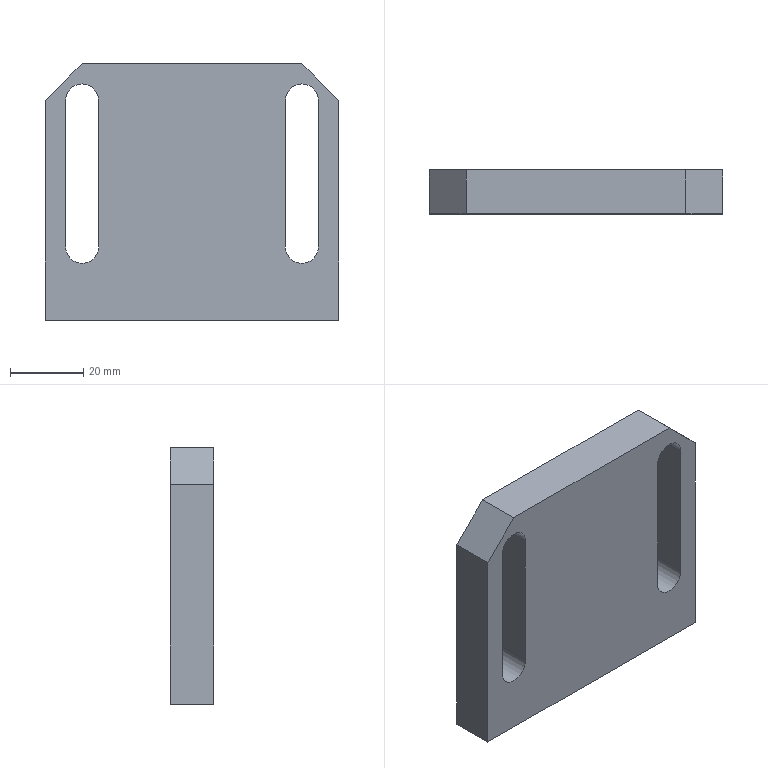Part | SolidWorks | features BaseBody 1 | 1 solid | 30 faces | box 80 x 12 x 70 mm | volume 54802 mm3 | cylinder 12 | plane 12 | cone 6 | commonest cylinder face diameters 5 x6 9 x6
STEP:
#1=CARTESIAN_POINT('',(30.,0.,29.5));
#2=VERTEX_POINT('',#1);
#3=CARTESIAN_POINT('',(34.5,0.,25.));
#4=VERTEX_POINT('',#3);
#5=CARTESIAN_POINT('',(30.,0.,25.));
#6=DIRECTION('',(0.,1.,0.));
#7=DIRECTION('',(0.,0.,-1.));
#8=AXIS2_PLACEMENT_3D('',#5,#6,#7);
#9=CIRCLE('',#8,4.5);
#10=EDGE_CURVE('',#2,#4,#9,.T.);
#11=ORIENTED_EDGE('',*,*,#10,.F.);
#12=CARTESIAN_POINT('',(30.,12.,29.5));
#13=VERTEX_POINT('',#12);
#14=CARTESIAN_POINT('',(30.,0.,29.5));
#15=DIRECTION('',(0.,1.,0.));
#16=VECTOR('',#15,1000.);
#17=LINE('',#14,#16);
#18=EDGE_CURVE('',#2,#13,#17,.T.);
#19=ORIENTED_EDGE('',*,*,#18,.T.);
#20=CARTESIAN_POINT('',(34.5,12.,25.));
#21=VERTEX_POINT('',#20);
#22=CARTESIAN_POINT('',(30.,12.,25.));
#23=DIRECTION('',(0.,1.,0.));
#24=DIRECTION('',(0.,0.,-1.));
#25=AXIS2_PLACEMENT_3D('',#22,#23,#24);
#26=CIRCLE('',#25,4.5);
#27=EDGE_CURVE('',#13,#21,#26,.T.);
#28=ORIENTED_EDGE('',*,*,#27,.T.);
#29=CARTESIAN_POINT('',(34.5,0.,25.));
#30=DIRECTION('',(0.,1.,0.));
#31=VECTOR('',#30,1000.);
#32=LINE('',#29,#31);
#33=EDGE_CURVE('',#4,#21,#32,.T.);
#34=ORIENTED_EDGE('',*,*,#33,.F.);
#35=EDGE_LOOP('',(#11,#19,#28,#34));
#36=FACE_OUTER_BOUND('',#35,.T.);
#37=CARTESIAN_POINT('',(30.,0.,25.));
#38=DIRECTION('',(0.,1.,0.));
#39=DIRECTION('',(0.,0.,1.));
#40=AXIS2_PLACEMENT_3D('',#37,#38,#39);
#41=CYLINDRICAL_SURFACE('',#40,4.5);
#42=ADVANCED_FACE('',(#36),#41,.F.);
#43=CARTESIAN_POINT('',(-30.,0.,29.5));
#44=VERTEX_POINT('',#43);
#45=CARTESIAN_POINT('',(-25.5,0.,25.));
#46=VERTEX_POINT('',#45);
#47=CARTESIAN_POINT('',(-30.,0.,25.));
#48=DIRECTION('',(0.,1.,0.));
#49=DIRECTION('',(0.,0.,1.));
#50=AXIS2_PLACEMENT_3D('',#47,#48,#49);
#51=CIRCLE('',#50,4.5);
#52=EDGE_CURVE('',#44,#46,#51,.T.);
#53=ORIENTED_EDGE('',*,*,#52,.F.);
#54=CARTESIAN_POINT('',(-30.,12.,29.5));
#55=VERTEX_POINT('',#54);
#56=CARTESIAN_POINT('',(-30.,0.,29.5));
#57=DIRECTION('',(0.,1.,0.));
#58=VECTOR('',#57,1000.);
#59=LINE('',#56,#58);
#60=EDGE_CURVE('',#44,#55,#59,.T.);
#61=ORIENTED_EDGE('',*,*,#60,.T.);
#62=CARTESIAN_POINT('',(-25.5,12.,25.));
#63=VERTEX_POINT('',#62);
#64=CARTESIAN_POINT('',(-30.,12.,25.));
#65=DIRECTION('',(0.,1.,0.));
#66=DIRECTION('',(0.,0.,1.));
#67=AXIS2_PLACEMENT_3D('',#64,#65,#66);
#68=CIRCLE('',#67,4.5);
#69=EDGE_CURVE('',#55,#63,#68,.T.);
#70=ORIENTED_EDGE('',*,*,#69,.T.);
#71=CARTESIAN_POINT('',(-25.5,0.,25.));
#72=DIRECTION('',(0.,1.,0.));
#73=VECTOR('',#72,1000.);
#74=LINE('',#71,#73);
#75=EDGE_CURVE('',#46,#63,#74,.T.);
#76=ORIENTED_EDGE('',*,*,#75,.F.);
#77=EDGE_LOOP('',(#53,#61,#70,#76));
#78=FACE_OUTER_BOUND('',#77,.T.);
#79=CARTESIAN_POINT('',(-30.,0.,25.));
#80=DIRECTION('',(0.,1.,0.));
#81=DIRECTION('',(0.,0.,1.));
#82=AXIS2_PLACEMENT_3D('',#79,#80,#81);
#83=CYLINDRICAL_SURFACE('',#82,4.5);
#84=ADVANCED_FACE('',(#78),#83,.F.);
#85=CARTESIAN_POINT('',(22.5,6.,-18.));
#86=VERTEX_POINT('',#85);
#87=CARTESIAN_POINT('',(17.5,6.,-18.));
#88=VERTEX_POINT('',#87);
#89=CARTESIAN_POINT('',(20.,6.,-18.));
#90=DIRECTION('',(0.,0.,-1.));
#91=DIRECTION('',(-1.,0.,0.));
#92=AXIS2_PLACEMENT_3D('',#89,#90,#91);
#93=CIRCLE('',#92,2.5);
#94=EDGE_CURVE('',#86,#88,#93,.T.);
#95=ORIENTED_EDGE('',*,*,#94,.F.);
#96=CARTESIAN_POINT('',(22.5,6.,-35.));
#97=VERTEX_POINT('',#96);
#98=CARTESIAN_POINT('',(22.5,6.,-35.));
#99=DIRECTION('',(0.,0.,-1.));
#100=VECTOR('',#99,1000.);
#101=LINE('',#98,#100);
#102=EDGE_CURVE('',#86,#97,#101,.T.);
#103=ORIENTED_EDGE('',*,*,#102,.T.);
#104=CARTESIAN_POINT('',(17.5,6.,-35.));
#105=VERTEX_POINT('',#104);
#106=CARTESIAN_POINT('',(20.,6.,-35.));
#107=DIRECTION('',(0.,0.,-1.));
#108=DIRECTION('',(-1.,0.,0.));
#109=AXIS2_PLACEMENT_3D('',#106,#107,#108);
#110=CIRCLE('',#109,2.5);
#111=EDGE_CURVE('',#97,#105,#110,.T.);
#112=ORIENTED_EDGE('',*,*,#111,.T.);
#113=CARTESIAN_POINT('',(17.5,6.,-35.));
#114=DIRECTION('',(0.,0.,-1.));
#115=VECTOR('',#114,1000.);
#116=LINE('',#113,#115);
#117=EDGE_CURVE('',#88,#105,#116,.T.);
#118=ORIENTED_EDGE('',*,*,#117,.F.);
#119=EDGE_LOOP('',(#95,#103,#112,#118));
#120=FACE_OUTER_BOUND('',#119,.T.);
#121=CARTESIAN_POINT('',(20.,6.,-35.));
#122=DIRECTION('',(0.,0.,-1.));
#123=DIRECTION('',(-1.,0.,0.));
#124=AXIS2_PLACEMENT_3D('',#121,#122,#123);
#125=CYLINDRICAL_SURFACE('',#124,2.5);
#126=ADVANCED_FACE('',(#120),#125,.F.);
#127=CARTESIAN_POINT('',(20.,6.,-16.498));
#128=VERTEX_POINT('',#127);
#129=CARTESIAN_POINT('',(17.5,6.,-18.));
#130=DIRECTION('',(-0.8572,0.,-0.515));
#131=VECTOR('',#130,1000.);
#132=LINE('',#129,#131);
#133=EDGE_CURVE('',#128,#88,#132,.T.);
#134=ORIENTED_EDGE('',*,*,#133,.F.);
#135=CARTESIAN_POINT('',(22.5,6.,-18.));
#136=DIRECTION('',(0.8572,0.,-0.515));
#137=VECTOR('',#136,1000.);
#138=LINE('',#135,#137);
#139=EDGE_CURVE('',#128,#86,#138,.T.);
#140=ORIENTED_EDGE('',*,*,#139,.T.);
#141=ORIENTED_EDGE('',*,*,#94,.T.);
#142=EDGE_LOOP('',(#134,#140,#141));
#143=FACE_OUTER_BOUND('',#142,.T.);
#144=CARTESIAN_POINT('',(20.,6.,-18.));
#145=DIRECTION('',(0.,0.,-1.));
#146=DIRECTION('',(-1.,0.,0.));
#147=AXIS2_PLACEMENT_3D('',#144,#145,#146);
#148=CONICAL_SURFACE('',#147,2.5,1.03);
#149=ADVANCED_FACE('',(#143),#148,.F.);
#150=CARTESIAN_POINT('',(2.5,6.,-18.));
#151=VERTEX_POINT('',#150);
#152=CARTESIAN_POINT('',(-2.5,6.,-18.));
#153=VERTEX_POINT('',#152);
#154=CARTESIAN_POINT('',(0.,6.,-18.));
#155=DIRECTION('',(0.,0.,-1.));
#156=DIRECTION('',(-1.,0.,0.));
#157=AXIS2_PLACEMENT_3D('',#154,#155,#156);
#158=CIRCLE('',#157,2.5);
#159=EDGE_CURVE('',#151,#153,#158,.T.);
#160=ORIENTED_EDGE('',*,*,#159,.F.);
#161=CARTESIAN_POINT('',(2.5,6.,-35.));
#162=VERTEX_POINT('',#161);
#163=CARTESIAN_POINT('',(2.5,6.,-35.));
#164=DIRECTION('',(0.,0.,-1.));
#165=VECTOR('',#164,1000.);
#166=LINE('',#163,#165);
#167=EDGE_CURVE('',#151,#162,#166,.T.);
#168=ORIENTED_EDGE('',*,*,#167,.T.);
#169=CARTESIAN_POINT('',(-2.5,6.,-35.));
#170=VERTEX_POINT('',#169);
#171=CARTESIAN_POINT('',(0.,6.,-35.));
#172=DIRECTION('',(0.,0.,-1.));
#173=DIRECTION('',(-1.,0.,0.));
#174=AXIS2_PLACEMENT_3D('',#171,#172,#173);
#175=CIRCLE('',#174,2.5);
#176=EDGE_CURVE('',#162,#170,#175,.T.);
#177=ORIENTED_EDGE('',*,*,#176,.T.);
#178=CARTESIAN_POINT('',(-2.5,6.,-35.));
#179=DIRECTION('',(0.,0.,-1.));
#180=VECTOR('',#179,1000.);
#181=LINE('',#178,#180);
#182=EDGE_CURVE('',#153,#170,#181,.T.);
#183=ORIENTED_EDGE('',*,*,#182,.F.);
#184=EDGE_LOOP('',(#160,#168,#177,#183));
#185=FACE_OUTER_BOUND('',#184,.T.);
#186=CARTESIAN_POINT('',(0.,6.,-35.));
#187=DIRECTION('',(0.,0.,-1.));
#188=DIRECTION('',(-1.,0.,0.));
#189=AXIS2_PLACEMENT_3D('',#186,#187,#188);
#190=CYLINDRICAL_SURFACE('',#189,2.5);
#191=ADVANCED_FACE('',(#185),#190,.F.);
#192=CARTESIAN_POINT('',(0.,6.,-16.498));
#193=VERTEX_POINT('',#192);
#194=CARTESIAN_POINT('',(-2.5,6.,-18.));
#195=DIRECTION('',(-0.8572,0.,-0.515));
#196=VECTOR('',#195,1000.);
#197=LINE('',#194,#196);
#198=EDGE_CURVE('',#193,#153,#197,.T.);
#199=ORIENTED_EDGE('',*,*,#198,.F.);
#200=CARTESIAN_POINT('',(2.5,6.,-18.));
#201=DIRECTION('',(0.8572,0.,-0.515));
#202=VECTOR('',#201,1000.);
#203=LINE('',#200,#202);
#204=EDGE_CURVE('',#193,#151,#203,.T.);
#205=ORIENTED_EDGE('',*,*,#204,.T.);
#206=ORIENTED_EDGE('',*,*,#159,.T.);
#207=EDGE_LOOP('',(#199,#205,#206));
#208=FACE_OUTER_BOUND('',#207,.T.);
#209=CARTESIAN_POINT('',(0.,6.,-18.));
#210=DIRECTION('',(0.,0.,-1.));
#211=DIRECTION('',(-1.,0.,0.));
#212=AXIS2_PLACEMENT_3D('',#209,#210,#211);
#213=CONICAL_SURFACE('',#212,2.5,1.03);
#214=ADVANCED_FACE('',(#208),#213,.F.);
#215=CARTESIAN_POINT('',(-17.5,6.,-18.));
#216=VERTEX_POINT('',#215);
#217=CARTESIAN_POINT('',(-22.5,6.,-18.));
#218=VERTEX_POINT('',#217);
#219=CARTESIAN_POINT('',(-20.,6.,-18.));
#220=DIRECTION('',(0.,0.,-1.));
#221=DIRECTION('',(-1.,0.,0.));
#222=AXIS2_PLACEMENT_3D('',#219,#220,#221);
#223=CIRCLE('',#222,2.5);
#224=EDGE_CURVE('',#216,#218,#223,.T.);
#225=ORIENTED_EDGE('',*,*,#224,.F.);
#226=CARTESIAN_POINT('',(-17.5,6.,-35.));
#227=VERTEX_POINT('',#226);
#228=CARTESIAN_POINT('',(-17.5,6.,-35.));
#229=DIRECTION('',(0.,0.,-1.));
#230=VECTOR('',#229,1000.);
#231=LINE('',#228,#230);
#232=EDGE_CURVE('',#216,#227,#231,.T.);
#233=ORIENTED_EDGE('',*,*,#232,.T.);
#234=CARTESIAN_POINT('',(-22.5,6.,-35.));
#235=VERTEX_POINT('',#234);
#236=CARTESIAN_POINT('',(-20.,6.,-35.));
#237=DIRECTION('',(0.,0.,-1.));
#238=DIRECTION('',(-1.,0.,0.));
#239=AXIS2_PLACEMENT_3D('',#236,#237,#238);
#240=CIRCLE('',#239,2.5);
#241=EDGE_CURVE('',#227,#235,#240,.T.);
#242=ORIENTED_EDGE('',*,*,#241,.T.);
#243=CARTESIAN_POINT('',(-22.5,6.,-35.));
#244=DIRECTION('',(0.,0.,-1.));
#245=VECTOR('',#244,1000.);
#246=LINE('',#243,#245);
#247=EDGE_CURVE('',#218,#235,#246,.T.);
#248=ORIENTED_EDGE('',*,*,#247,.F.);
#249=EDGE_LOOP('',(#225,#233,#242,#248));
#250=FACE_OUTER_BOUND('',#249,.T.);
#251=CARTESIAN_POINT('',(-20.,6.,-35.));
#252=DIRECTION('',(0.,0.,-1.));
#253=DIRECTION('',(-1.,0.,0.));
#254=AXIS2_PLACEMENT_3D('',#251,#252,#253);
#255=CYLINDRICAL_SURFACE('',#254,2.5);
#256=ADVANCED_FACE('',(#250),#255,.F.);
#257=CARTESIAN_POINT('',(-20.,6.,-16.498));
#258=VERTEX_POINT('',#257);
#259=CARTESIAN_POINT('',(-22.5,6.,-18.));
#260=DIRECTION('',(-0.8572,0.,-0.515));
#261=VECTOR('',#260,1000.);
#262=LINE('',#259,#261);
#263=EDGE_CURVE('',#258,#218,#262,.T.);
#264=ORIENTED_EDGE('',*,*,#263,.F.);
#265=CARTESIAN_POINT('',(-17.5,6.,-18.));
#266=DIRECTION('',(0.8572,0.,-0.515));
#267=VECTOR('',#266,1000.);
#268=LINE('',#265,#267);
#269=EDGE_CURVE('',#258,#216,#268,.T.);
#270=ORIENTED_EDGE('',*,*,#269,.T.);
#271=ORIENTED_EDGE('',*,*,#224,.T.);
#272=EDGE_LOOP('',(#264,#270,#271));
#273=FACE_OUTER_BOUND('',#272,.T.);
#274=CARTESIAN_POINT('',(-20.,6.,-18.));
#275=DIRECTION('',(0.,0.,-1.));
#276=DIRECTION('',(-1.,0.,0.));
#277=AXIS2_PLACEMENT_3D('',#274,#275,#276);
#278=CONICAL_SURFACE('',#277,2.5,1.03);
#279=ADVANCED_FACE('',(#273),#278,.F.);
#280=CARTESIAN_POINT('',(-40.,0.,-35.));
#281=VERTEX_POINT('',#280);
#282=CARTESIAN_POINT('',(-40.,0.,25.));
#283=VERTEX_POINT('',#282);
#284=CARTESIAN_POINT('',(-40.,0.,-35.));
#285=DIRECTION('',(0.,0.,1.));
#286=VECTOR('',#285,1000.);
#287=LINE('',#284,#286);
#288=EDGE_CURVE('',#281,#283,#287,.T.);
#289=ORIENTED_EDGE('',*,*,#288,.T.);
#290=CARTESIAN_POINT('',(-40.,12.,25.));
#291=VERTEX_POINT('',#290);
#292=CARTESIAN_POINT('',(-40.,12.,25.));
#293=DIRECTION('',(0.,1.,0.));
#294=VECTOR('',#293,1000.);
#295=LINE('',#292,#294);
#296=EDGE_CURVE('',#283,#291,#295,.T.);
#297=ORIENTED_EDGE('',*,*,#296,.T.);
#298=CARTESIAN_POINT('',(-40.,12.,-35.));
#299=VERTEX_POINT('',#298);
#300=CARTESIAN_POINT('',(-40.,12.,-35.));
#301=DIRECTION('',(0.,0.,1.));
#302=VECTOR('',#301,1000.);
#303=LINE('',#300,#302);
#304=EDGE_CURVE('',#299,#291,#303,.T.);
#305=ORIENTED_EDGE('',*,*,#304,.F.);
#306=CARTESIAN_POINT('',(-40.,12.,-35.));
#307=DIRECTION('',(0.,-1.,0.));
#308=VECTOR('',#307,1000.);
#309=LINE('',#306,#308);
#310=EDGE_CURVE('',#299,#281,#309,.T.);
#311=ORIENTED_EDGE('',*,*,#310,.T.);
#312=EDGE_LOOP('',(#289,#297,#305,#311));
#313=FACE_OUTER_BOUND('',#312,.T.);
#314=CARTESIAN_POINT('',(-40.,12.,-35.));
#315=DIRECTION('',(1.,0.,0.));
#316=DIRECTION('',(0.,0.,-1.));
#317=AXIS2_PLACEMENT_3D('',#314,#315,#316);
#318=PLANE('',#317);
#319=ADVANCED_FACE('',(#313),#318,.F.);
#320=CARTESIAN_POINT('',(-30.,0.,35.));
#321=VERTEX_POINT('',#320);
#322=CARTESIAN_POINT('',(30.,0.,35.));
#323=VERTEX_POINT('',#322);
#324=CARTESIAN_POINT('',(40.,0.,35.));
#325=DIRECTION('',(1.,0.,0.));
#326=VECTOR('',#325,1000.);
#327=LINE('',#324,#326);
#328=EDGE_CURVE('',#321,#323,#327,.T.);
#329=ORIENTED_EDGE('',*,*,#328,.T.);
#330=CARTESIAN_POINT('',(30.,12.,35.));
#331=VERTEX_POINT('',#330);
#332=CARTESIAN_POINT('',(30.,12.,35.));
#333=DIRECTION('',(0.,1.,0.));
#334=VECTOR('',#333,1000.);
#335=LINE('',#332,#334);
#336=EDGE_CURVE('',#323,#331,#335,.T.);
#337=ORIENTED_EDGE('',*,*,#336,.T.);
#338=CARTESIAN_POINT('',(-30.,12.,35.));
#339=VERTEX_POINT('',#338);
#340=CARTESIAN_POINT('',(40.,12.,35.));
#341=DIRECTION('',(1.,0.,0.));
#342=VECTOR('',#341,1000.);
#343=LINE('',#340,#342);
#344=EDGE_CURVE('',#339,#331,#343,.T.);
#345=ORIENTED_EDGE('',*,*,#344,.F.);
#346=CARTESIAN_POINT('',(-30.,12.,35.));
#347=DIRECTION('',(0.,-1.,0.));
#348=VECTOR('',#347,1000.);
#349=LINE('',#346,#348);
#350=EDGE_CURVE('',#339,#321,#349,.T.);
#351=ORIENTED_EDGE('',*,*,#350,.T.);
#352=EDGE_LOOP('',(#329,#337,#345,#351));
#353=FACE_OUTER_BOUND('',#352,.T.);
#354=CARTESIAN_POINT('',(40.,12.,35.));
#355=DIRECTION('',(0.,0.,-1.));
#356=DIRECTION('',(-1.,0.,0.));
#357=AXIS2_PLACEMENT_3D('',#354,#355,#356);
#358=PLANE('',#357);
#359=ADVANCED_FACE('',(#353),#358,.F.);
#360=CARTESIAN_POINT('',(40.,12.,25.));
#361=VERTEX_POINT('',#360);
#362=CARTESIAN_POINT('',(40.,12.,-35.));
#363=VERTEX_POINT('',#362);
#364=CARTESIAN_POINT('',(40.,12.,-35.));
#365=DIRECTION('',(0.,0.,-1.));
#366=VECTOR('',#365,1000.);
#367=LINE('',#364,#366);
#368=EDGE_CURVE('',#361,#363,#367,.T.);
#369=ORIENTED_EDGE('',*,*,#368,.F.);
#370=CARTESIAN_POINT('',(40.,0.,25.));
#371=VERTEX_POINT('',#370);
#372=CARTESIAN_POINT('',(40.,12.,25.));
#373=DIRECTION('',(0.,-1.,0.));
#374=VECTOR('',#373,1000.);
#375=LINE('',#372,#374);
#376=EDGE_CURVE('',#361,#371,#375,.T.);
#377=ORIENTED_EDGE('',*,*,#376,.T.);
#378=CARTESIAN_POINT('',(40.,0.,-35.));
#379=VERTEX_POINT('',#378);
#380=CARTESIAN_POINT('',(40.,0.,-35.));
#381=DIRECTION('',(0.,0.,-1.));
#382=VECTOR('',#381,1000.);
#383=LINE('',#380,#382);
#384=EDGE_CURVE('',#371,#379,#383,.T.);
#385=ORIENTED_EDGE('',*,*,#384,.T.);
#386=CARTESIAN_POINT('',(40.,12.,-35.));
#387=DIRECTION('',(0.,-1.,0.));
#388=VECTOR('',#387,1000.);
#389=LINE('',#386,#388);
#390=EDGE_CURVE('',#363,#379,#389,.T.);
#391=ORIENTED_EDGE('',*,*,#390,.F.);
#392=EDGE_LOOP('',(#369,#377,#385,#391));
#393=FACE_OUTER_BOUND('',#392,.T.);
#394=CARTESIAN_POINT('',(40.,12.,-35.));
#395=DIRECTION('',(-1.,0.,0.));
#396=DIRECTION('',(0.,0.,1.));
#397=AXIS2_PLACEMENT_3D('',#394,#395,#396);
#398=PLANE('',#397);
#399=ADVANCED_FACE('',(#393),#398,.F.);
#400=CARTESIAN_POINT('',(20.,6.,-35.));
#401=DIRECTION('',(0.,0.,-1.));
#402=DIRECTION('',(-1.,0.,0.));
#403=AXIS2_PLACEMENT_3D('',#400,#401,#402);
#404=CIRCLE('',#403,2.5);
#405=EDGE_CURVE('',#105,#97,#404,.T.);
#406=ORIENTED_EDGE('',*,*,#405,.F.);
#407=ORIENTED_EDGE('',*,*,#111,.F.);
#408=EDGE_LOOP('',(#406,#407));
#409=FACE_BOUND('',#408,.T.);
#410=CARTESIAN_POINT('',(0.,6.,-35.));
#411=DIRECTION('',(0.,0.,-1.));
#412=DIRECTION('',(-1.,0.,0.));
#413=AXIS2_PLACEMENT_3D('',#410,#411,#412);
#414=CIRCLE('',#413,2.5);
#415=EDGE_CURVE('',#170,#162,#414,.T.);
#416=ORIENTED_EDGE('',*,*,#415,.F.);
#417=ORIENTED_EDGE('',*,*,#176,.F.);
#418=EDGE_LOOP('',(#416,#417));
#419=FACE_BOUND('',#418,.T.);
#420=CARTESIAN_POINT('',(-20.,6.,-35.));
#421=DIRECTION('',(0.,0.,-1.));
#422=DIRECTION('',(-1.,0.,0.));
#423=AXIS2_PLACEMENT_3D('',#420,#421,#422);
#424=CIRCLE('',#423,2.5);
#425=EDGE_CURVE('',#235,#227,#424,.T.);
#426=ORIENTED_EDGE('',*,*,#425,.F.);
#427=ORIENTED_EDGE('',*,*,#241,.F.);
#428=EDGE_LOOP('',(#426,#427));
#429=FACE_BOUND('',#428,.T.);
#430=CARTESIAN_POINT('',(40.,0.,-35.));
#431=DIRECTION('',(-1.,0.,0.));
#432=VECTOR('',#431,1000.);
#433=LINE('',#430,#432);
#434=EDGE_CURVE('',#379,#281,#433,.T.);
#435=ORIENTED_EDGE('',*,*,#434,.T.);
#436=ORIENTED_EDGE('',*,*,#310,.F.);
#437=CARTESIAN_POINT('',(40.,12.,-35.));
#438=DIRECTION('',(-1.,0.,0.));
#439=VECTOR('',#438,1000.);
#440=LINE('',#437,#439);
#441=EDGE_CURVE('',#363,#299,#440,.T.);
#442=ORIENTED_EDGE('',*,*,#441,.F.);
#443=ORIENTED_EDGE('',*,*,#390,.T.);
#444=EDGE_LOOP('',(#435,#436,#442,#443));
#445=FACE_OUTER_BOUND('',#444,.T.);
#446=CARTESIAN_POINT('',(40.,12.,-35.));
#447=DIRECTION('',(0.,0.,1.));
#448=DIRECTION('',(1.,0.,0.));
#449=AXIS2_PLACEMENT_3D('',#446,#447,#448);
#450=PLANE('',#449);
#451=ADVANCED_FACE('',(#409,#419,#429,#445),#450,.F.);
#452=CARTESIAN_POINT('',(25.5,12.,-15.));
#453=VERTEX_POINT('',#452);
#454=CARTESIAN_POINT('',(25.5,12.,25.));
#455=VERTEX_POINT('',#454);
#456=CARTESIAN_POINT('',(25.5,12.,-15.));
#457=DIRECTION('',(0.,0.,1.));
#458=VECTOR('',#457,1000.);
#459=LINE('',#456,#458);
#460=EDGE_CURVE('',#453,#455,#459,.T.);
#461=ORIENTED_EDGE('',*,*,#460,.F.);
#462=CARTESIAN_POINT('',(34.5,12.,-15.));
#463=VERTEX_POINT('',#462);
#464=CARTESIAN_POINT('',(30.,12.,-15.));
#465=DIRECTION('',(0.,1.,0.));
#466=DIRECTION('',(0.,0.,-1.));
#467=AXIS2_PLACEMENT_3D('',#464,#465,#466);
#468=CIRCLE('',#467,4.5);
#469=EDGE_CURVE('',#463,#453,#468,.T.);
#470=ORIENTED_EDGE('',*,*,#469,.F.);
#471=CARTESIAN_POINT('',(34.5,12.,-15.));
#472=DIRECTION('',(0.,0.,-1.));
#473=VECTOR('',#472,1000.);
#474=LINE('',#471,#473);
#475=EDGE_CURVE('',#21,#463,#474,.T.);
#476=ORIENTED_EDGE('',*,*,#475,.F.);
#477=ORIENTED_EDGE('',*,*,#27,.F.);
#478=CARTESIAN_POINT('',(30.,12.,25.));
#479=DIRECTION('',(0.,1.,0.));
#480=DIRECTION('',(0.,0.,-1.));
#481=AXIS2_PLACEMENT_3D('',#478,#479,#480);
#482=CIRCLE('',#481,4.5);
#483=EDGE_CURVE('',#455,#13,#482,.T.);
#484=ORIENTED_EDGE('',*,*,#483,.F.);
#485=EDGE_LOOP('',(#461,#470,#476,#477,#484));
#486=FACE_BOUND('',#485,.T.);
#487=CARTESIAN_POINT('',(-34.5,12.,-15.));
#488=VERTEX_POINT('',#487);
#489=CARTESIAN_POINT('',(-34.5,12.,25.));
#490=VERTEX_POINT('',#489);
#491=CARTESIAN_POINT('',(-34.5,12.,-15.));
#492=DIRECTION('',(0.,0.,1.));
#493=VECTOR('',#492,1000.);
#494=LINE('',#491,#493);
#495=EDGE_CURVE('',#488,#490,#494,.T.);
#496=ORIENTED_EDGE('',*,*,#495,.F.);
#497=CARTESIAN_POINT('',(-25.5,12.,-15.));
#498=VERTEX_POINT('',#497);
#499=CARTESIAN_POINT('',(-30.,12.,-15.));
#500=DIRECTION('',(0.,1.,0.));
#501=DIRECTION('',(0.,0.,1.));
#502=AXIS2_PLACEMENT_3D('',#499,#500,#501);
#503=CIRCLE('',#502,4.5);
#504=EDGE_CURVE('',#498,#488,#503,.T.);
#505=ORIENTED_EDGE('',*,*,#504,.F.);
#506=CARTESIAN_POINT('',(-25.5,12.,-15.));
#507=DIRECTION('',(0.,0.,-1.));
#508=VECTOR('',#507,1000.);
#509=LINE('',#506,#508);
#510=EDGE_CURVE('',#63,#498,#509,.T.);
#511=ORIENTED_EDGE('',*,*,#510,.F.);
#512=ORIENTED_EDGE('',*,*,#69,.F.);
#513=CARTESIAN_POINT('',(-30.,12.,25.));
#514=DIRECTION('',(0.,1.,0.));
#515=DIRECTION('',(0.,0.,1.));
#516=AXIS2_PLACEMENT_3D('',#513,#514,#515);
#517=CIRCLE('',#516,4.5);
#518=EDGE_CURVE('',#490,#55,#517,.T.);
#519=ORIENTED_EDGE('',*,*,#518,.F.);
#520=EDGE_LOOP('',(#496,#505,#511,#512,#519));
#521=FACE_BOUND('',#520,.T.);
#522=ORIENTED_EDGE('',*,*,#344,.T.);
#523=CARTESIAN_POINT('',(40.,12.,25.));
#524=DIRECTION('',(0.7071,0.,-0.7071));
#525=VECTOR('',#524,1000.);
#526=LINE('',#523,#525);
#527=EDGE_CURVE('',#331,#361,#526,.T.);
#528=ORIENTED_EDGE('',*,*,#527,.T.);
#529=ORIENTED_EDGE('',*,*,#368,.T.);
#530=ORIENTED_EDGE('',*,*,#441,.T.);
#531=ORIENTED_EDGE('',*,*,#304,.T.);
#532=CARTESIAN_POINT('',(-30.,12.,35.));
#533=DIRECTION('',(0.7071,0.,0.7071));
#534=VECTOR('',#533,1000.);
#535=LINE('',#532,#534);
#536=EDGE_CURVE('',#291,#339,#535,.T.);
#537=ORIENTED_EDGE('',*,*,#536,.T.);
#538=EDGE_LOOP('',(#522,#528,#529,#530,#531,#537));
#539=FACE_OUTER_BOUND('',#538,.T.);
#540=CARTESIAN_POINT('',(0.,12.,0.));
#541=DIRECTION('',(0.,-1.,0.));
#542=DIRECTION('',(0.,0.,-1.));
#543=AXIS2_PLACEMENT_3D('',#540,#541,#542);
#544=PLANE('',#543);
#545=ADVANCED_FACE('',(#486,#521,#539),#544,.F.);
#546=CARTESIAN_POINT('',(34.5,0.,-15.));
#547=VERTEX_POINT('',#546);
#548=CARTESIAN_POINT('',(25.5,0.,-15.));
#549=VERTEX_POINT('',#548);
#550=CARTESIAN_POINT('',(30.,0.,-15.));
#551=DIRECTION('',(0.,1.,0.));
#552=DIRECTION('',(0.,0.,-1.));
#553=AXIS2_PLACEMENT_3D('',#550,#551,#552);
#554=CIRCLE('',#553,4.5);
#555=EDGE_CURVE('',#547,#549,#554,.T.);
#556=ORIENTED_EDGE('',*,*,#555,.T.);
#557=CARTESIAN_POINT('',(25.5,0.,25.));
#558=VERTEX_POINT('',#557);
#559=CARTESIAN_POINT('',(25.5,0.,-15.));
#560=DIRECTION('',(0.,0.,1.));
#561=VECTOR('',#560,1000.);
#562=LINE('',#559,#561);
#563=EDGE_CURVE('',#549,#558,#562,.T.);
#564=ORIENTED_EDGE('',*,*,#563,.T.);
#565=CARTESIAN_POINT('',(30.,0.,25.));
#566=DIRECTION('',(0.,1.,0.));
#567=DIRECTION('',(0.,0.,-1.));
#568=AXIS2_PLACEMENT_3D('',#565,#566,#567);
#569=CIRCLE('',#568,4.5);
#570=EDGE_CURVE('',#558,#2,#569,.T.);
#571=ORIENTED_EDGE('',*,*,#570,.T.);
#572=ORIENTED_EDGE('',*,*,#10,.T.);
#573=CARTESIAN_POINT('',(34.5,0.,-15.));
#574=DIRECTION('',(0.,0.,-1.));
#575=VECTOR('',#574,1000.);
#576=LINE('',#573,#575);
#577=EDGE_CURVE('',#4,#547,#576,.T.);
#578=ORIENTED_EDGE('',*,*,#577,.T.);
#579=EDGE_LOOP('',(#556,#564,#571,#572,#578));
#580=FACE_BOUND('',#579,.T.);
#581=CARTESIAN_POINT('',(-25.5,0.,-15.));
#582=VERTEX_POINT('',#581);
#583=CARTESIAN_POINT('',(-34.5,0.,-15.));
#584=VERTEX_POINT('',#583);
#585=CARTESIAN_POINT('',(-30.,0.,-15.));
#586=DIRECTION('',(0.,1.,0.));
#587=DIRECTION('',(0.,0.,1.));
#588=AXIS2_PLACEMENT_3D('',#585,#586,#587);
#589=CIRCLE('',#588,4.5);
#590=EDGE_CURVE('',#582,#584,#589,.T.);
#591=ORIENTED_EDGE('',*,*,#590,.T.);
#592=CARTESIAN_POINT('',(-34.5,0.,25.));
#593=VERTEX_POINT('',#592);
#594=CARTESIAN_POINT('',(-34.5,0.,-15.));
#595=DIRECTION('',(0.,0.,1.));
#596=VECTOR('',#595,1000.);
#597=LINE('',#594,#596);
#598=EDGE_CURVE('',#584,#593,#597,.T.);
#599=ORIENTED_EDGE('',*,*,#598,.T.);
#600=CARTESIAN_POINT('',(-30.,0.,25.));
#601=DIRECTION('',(0.,1.,0.));
#602=DIRECTION('',(0.,0.,1.));
#603=AXIS2_PLACEMENT_3D('',#600,#601,#602);
#604=CIRCLE('',#603,4.5);
#605=EDGE_CURVE('',#593,#44,#604,.T.);
#606=ORIENTED_EDGE('',*,*,#605,.T.);
#607=ORIENTED_EDGE('',*,*,#52,.T.);
#608=CARTESIAN_POINT('',(-25.5,0.,-15.));
#609=DIRECTION('',(0.,0.,-1.));
#610=VECTOR('',#609,1000.);
#611=LINE('',#608,#610);
#612=EDGE_CURVE('',#46,#582,#611,.T.);
#613=ORIENTED_EDGE('',*,*,#612,.T.);
#614=EDGE_LOOP('',(#591,#599,#606,#607,#613));
#615=FACE_BOUND('',#614,.T.);
#616=ORIENTED_EDGE('',*,*,#384,.F.);
#617=CARTESIAN_POINT('',(32.5,0.,32.5));
#618=DIRECTION('',(-0.7071,0.,0.7071));
#619=VECTOR('',#618,1000.);
#620=LINE('',#617,#619);
#621=EDGE_CURVE('',#371,#323,#620,.T.);
#622=ORIENTED_EDGE('',*,*,#621,.T.);
#623=ORIENTED_EDGE('',*,*,#328,.F.);
#624=CARTESIAN_POINT('',(-32.5,0.,32.5));
#625=DIRECTION('',(-0.7071,0.,-0.7071));
#626=VECTOR('',#625,1000.);
#627=LINE('',#624,#626);
#628=EDGE_CURVE('',#321,#283,#627,.T.);
#629=ORIENTED_EDGE('',*,*,#628,.T.);
#630=ORIENTED_EDGE('',*,*,#288,.F.);
#631=ORIENTED_EDGE('',*,*,#434,.F.);
#632=EDGE_LOOP('',(#616,#622,#623,#629,#630,#631));
#633=FACE_OUTER_BOUND('',#632,.T.);
#634=CARTESIAN_POINT('',(0.,0.,0.));
#635=DIRECTION('',(0.,-1.,0.));
#636=DIRECTION('',(0.,0.,-1.));
#637=AXIS2_PLACEMENT_3D('',#634,#635,#636);
#638=PLANE('',#637);
#639=ADVANCED_FACE('',(#580,#615,#633),#638,.T.);
#640=ORIENTED_EDGE('',*,*,#269,.F.);
#641=ORIENTED_EDGE('',*,*,#263,.T.);
#642=CARTESIAN_POINT('',(-20.,6.,-18.));
#643=DIRECTION('',(0.,0.,-1.));
#644=DIRECTION('',(-1.,0.,0.));
#645=AXIS2_PLACEMENT_3D('',#642,#643,#644);
#646=CIRCLE('',#645,2.5);
#647=EDGE_CURVE('',#218,#216,#646,.T.);
#648=ORIENTED_EDGE('',*,*,#647,.T.);
#649=EDGE_LOOP('',(#640,#641,#648));
#650=FACE_OUTER_BOUND('',#649,.T.);
#651=CARTESIAN_POINT('',(-20.,6.,-18.));
#652=DIRECTION('',(0.,0.,-1.));
#653=DIRECTION('',(-1.,0.,0.));
#654=AXIS2_PLACEMENT_3D('',#651,#652,#653);
#655=CONICAL_SURFACE('',#654,2.5,1.03);
#656=ADVANCED_FACE('',(#650),#655,.F.);
#657=ORIENTED_EDGE('',*,*,#232,.F.);
#658=ORIENTED_EDGE('',*,*,#647,.F.);
#659=ORIENTED_EDGE('',*,*,#247,.T.);
#660=ORIENTED_EDGE('',*,*,#425,.T.);
#661=EDGE_LOOP('',(#657,#658,#659,#660));
#662=FACE_OUTER_BOUND('',#661,.T.);
#663=CARTESIAN_POINT('',(-20.,6.,-35.));
#664=DIRECTION('',(0.,0.,-1.));
#665=DIRECTION('',(-1.,0.,0.));
#666=AXIS2_PLACEMENT_3D('',#663,#664,#665);
#667=CYLINDRICAL_SURFACE('',#666,2.5);
#668=ADVANCED_FACE('',(#662),#667,.F.);
#669=ORIENTED_EDGE('',*,*,#204,.F.);
#670=ORIENTED_EDGE('',*,*,#198,.T.);
#671=CARTESIAN_POINT('',(0.,6.,-18.));
#672=DIRECTION('',(0.,0.,-1.));
#673=DIRECTION('',(-1.,0.,0.));
#674=AXIS2_PLACEMENT_3D('',#671,#672,#673);
#675=CIRCLE('',#674,2.5);
#676=EDGE_CURVE('',#153,#151,#675,.T.);
#677=ORIENTED_EDGE('',*,*,#676,.T.);
#678=EDGE_LOOP('',(#669,#670,#677));
#679=FACE_OUTER_BOUND('',#678,.T.);
#680=CARTESIAN_POINT('',(0.,6.,-18.));
#681=DIRECTION('',(0.,0.,-1.));
#682=DIRECTION('',(-1.,0.,0.));
#683=AXIS2_PLACEMENT_3D('',#680,#681,#682);
#684=CONICAL_SURFACE('',#683,2.5,1.03);
#685=ADVANCED_FACE('',(#679),#684,.F.);
#686=ORIENTED_EDGE('',*,*,#167,.F.);
#687=ORIENTED_EDGE('',*,*,#676,.F.);
#688=ORIENTED_EDGE('',*,*,#182,.T.);
#689=ORIENTED_EDGE('',*,*,#415,.T.);
#690=EDGE_LOOP('',(#686,#687,#688,#689));
#691=FACE_OUTER_BOUND('',#690,.T.);
#692=CARTESIAN_POINT('',(0.,6.,-35.));
#693=DIRECTION('',(0.,0.,-1.));
#694=DIRECTION('',(-1.,0.,0.));
#695=AXIS2_PLACEMENT_3D('',#692,#693,#694);
#696=CYLINDRICAL_SURFACE('',#695,2.5);
#697=ADVANCED_FACE('',(#691),#696,.F.);
#698=ORIENTED_EDGE('',*,*,#139,.F.);
#699=ORIENTED_EDGE('',*,*,#133,.T.);
#700=CARTESIAN_POINT('',(20.,6.,-18.));
#701=DIRECTION('',(0.,0.,-1.));
#702=DIRECTION('',(-1.,0.,0.));
#703=AXIS2_PLACEMENT_3D('',#700,#701,#702);
#704=CIRCLE('',#703,2.5);
#705=EDGE_CURVE('',#88,#86,#704,.T.);
#706=ORIENTED_EDGE('',*,*,#705,.T.);
#707=EDGE_LOOP('',(#698,#699,#706));
#708=FACE_OUTER_BOUND('',#707,.T.);
#709=CARTESIAN_POINT('',(20.,6.,-18.));
#710=DIRECTION('',(0.,0.,-1.));
#711=DIRECTION('',(-1.,0.,0.));
#712=AXIS2_PLACEMENT_3D('',#709,#710,#711);
#713=CONICAL_SURFACE('',#712,2.5,1.03);
#714=ADVANCED_FACE('',(#708),#713,.F.);
#715=ORIENTED_EDGE('',*,*,#102,.F.);
#716=ORIENTED_EDGE('',*,*,#705,.F.);
#717=ORIENTED_EDGE('',*,*,#117,.T.);
#718=ORIENTED_EDGE('',*,*,#405,.T.);
#719=EDGE_LOOP('',(#715,#716,#717,#718));
#720=FACE_OUTER_BOUND('',#719,.T.);
#721=CARTESIAN_POINT('',(20.,6.,-35.));
#722=DIRECTION('',(0.,0.,-1.));
#723=DIRECTION('',(-1.,0.,0.));
#724=AXIS2_PLACEMENT_3D('',#721,#722,#723);
#725=CYLINDRICAL_SURFACE('',#724,2.5);
#726=ADVANCED_FACE('',(#720),#725,.F.);
#727=ORIENTED_EDGE('',*,*,#527,.F.);
#728=ORIENTED_EDGE('',*,*,#336,.F.);
#729=ORIENTED_EDGE('',*,*,#621,.F.);
#730=ORIENTED_EDGE('',*,*,#376,.F.);
#731=EDGE_LOOP('',(#727,#728,#729,#730));
#732=FACE_OUTER_BOUND('',#731,.T.);
#733=CARTESIAN_POINT('',(40.,12.,25.));
#734=DIRECTION('',(-0.7071,0.,-0.7071));
#735=DIRECTION('',(0.,-1.,0.));
#736=AXIS2_PLACEMENT_3D('',#733,#734,#735);
#737=PLANE('',#736);
#738=ADVANCED_FACE('',(#732),#737,.F.);
#739=ORIENTED_EDGE('',*,*,#536,.F.);
#740=ORIENTED_EDGE('',*,*,#296,.F.);
#741=ORIENTED_EDGE('',*,*,#628,.F.);
#742=ORIENTED_EDGE('',*,*,#350,.F.);
#743=EDGE_LOOP('',(#739,#740,#741,#742));
#744=FACE_OUTER_BOUND('',#743,.T.);
#745=CARTESIAN_POINT('',(-30.,12.,35.));
#746=DIRECTION('',(0.7071,0.,-0.7071));
#747=DIRECTION('',(0.,-1.,0.));
#748=AXIS2_PLACEMENT_3D('',#745,#746,#747);
#749=PLANE('',#748);
#750=ADVANCED_FACE('',(#744),#749,.F.);
#751=ORIENTED_EDGE('',*,*,#504,.T.);
#752=CARTESIAN_POINT('',(-34.5,0.,-15.));
#753=DIRECTION('',(0.,1.,0.));
#754=VECTOR('',#753,1000.);
#755=LINE('',#752,#754);
#756=EDGE_CURVE('',#584,#488,#755,.T.);
#757=ORIENTED_EDGE('',*,*,#756,.F.);
#758=ORIENTED_EDGE('',*,*,#590,.F.);
#759=CARTESIAN_POINT('',(-25.5,0.,-15.));
#760=DIRECTION('',(0.,1.,0.));
#761=VECTOR('',#760,1000.);
#762=LINE('',#759,#761);
#763=EDGE_CURVE('',#582,#498,#762,.T.);
#764=ORIENTED_EDGE('',*,*,#763,.T.);
#765=EDGE_LOOP('',(#751,#757,#758,#764));
#766=FACE_OUTER_BOUND('',#765,.T.);
#767=CARTESIAN_POINT('',(-30.,0.,-15.));
#768=DIRECTION('',(0.,1.,0.));
#769=DIRECTION('',(0.,0.,1.));
#770=AXIS2_PLACEMENT_3D('',#767,#768,#769);
#771=CYLINDRICAL_SURFACE('',#770,4.5);
#772=ADVANCED_FACE('',(#766),#771,.F.);
#773=ORIENTED_EDGE('',*,*,#510,.T.);
#774=ORIENTED_EDGE('',*,*,#763,.F.);
#775=ORIENTED_EDGE('',*,*,#612,.F.);
#776=ORIENTED_EDGE('',*,*,#75,.T.);
#777=EDGE_LOOP('',(#773,#774,#775,#776));
#778=FACE_OUTER_BOUND('',#777,.T.);
#779=CARTESIAN_POINT('',(-25.5,0.,-15.));
#780=DIRECTION('',(1.,0.,0.));
#781=DIRECTION('',(0.,0.,-1.));
#782=AXIS2_PLACEMENT_3D('',#779,#780,#781);
#783=PLANE('',#782);
#784=ADVANCED_FACE('',(#778),#783,.F.);
#785=ORIENTED_EDGE('',*,*,#60,.F.);
#786=ORIENTED_EDGE('',*,*,#605,.F.);
#787=CARTESIAN_POINT('',(-34.5,0.,25.));
#788=DIRECTION('',(0.,1.,0.));
#789=VECTOR('',#788,1000.);
#790=LINE('',#787,#789);
#791=EDGE_CURVE('',#593,#490,#790,.T.);
#792=ORIENTED_EDGE('',*,*,#791,.T.);
#793=ORIENTED_EDGE('',*,*,#518,.T.);
#794=EDGE_LOOP('',(#785,#786,#792,#793));
#795=FACE_OUTER_BOUND('',#794,.T.);
#796=CARTESIAN_POINT('',(-30.,0.,25.));
#797=DIRECTION('',(0.,1.,0.));
#798=DIRECTION('',(0.,0.,1.));
#799=AXIS2_PLACEMENT_3D('',#796,#797,#798);
#800=CYLINDRICAL_SURFACE('',#799,4.5);
#801=ADVANCED_FACE('',(#795),#800,.F.);
#802=ORIENTED_EDGE('',*,*,#495,.T.);
#803=ORIENTED_EDGE('',*,*,#791,.F.);
#804=ORIENTED_EDGE('',*,*,#598,.F.);
#805=ORIENTED_EDGE('',*,*,#756,.T.);
#806=EDGE_LOOP('',(#802,#803,#804,#805));
#807=FACE_OUTER_BOUND('',#806,.T.);
#808=CARTESIAN_POINT('',(-34.5,0.,-15.));
#809=DIRECTION('',(-1.,0.,0.));
#810=DIRECTION('',(0.,0.,1.));
#811=AXIS2_PLACEMENT_3D('',#808,#809,#810);
#812=PLANE('',#811);
#813=ADVANCED_FACE('',(#807),#812,.F.);
#814=ORIENTED_EDGE('',*,*,#469,.T.);
#815=CARTESIAN_POINT('',(25.5,0.,-15.));
#816=DIRECTION('',(0.,1.,0.));
#817=VECTOR('',#816,1000.);
#818=LINE('',#815,#817);
#819=EDGE_CURVE('',#549,#453,#818,.T.);
#820=ORIENTED_EDGE('',*,*,#819,.F.);
#821=ORIENTED_EDGE('',*,*,#555,.F.);
#822=CARTESIAN_POINT('',(34.5,0.,-15.));
#823=DIRECTION('',(0.,1.,0.));
#824=VECTOR('',#823,1000.);
#825=LINE('',#822,#824);
#826=EDGE_CURVE('',#547,#463,#825,.T.);
#827=ORIENTED_EDGE('',*,*,#826,.T.);
#828=EDGE_LOOP('',(#814,#820,#821,#827));
#829=FACE_OUTER_BOUND('',#828,.T.);
#830=CARTESIAN_POINT('',(30.,0.,-15.));
#831=DIRECTION('',(0.,1.,0.));
#832=DIRECTION('',(0.,0.,1.));
#833=AXIS2_PLACEMENT_3D('',#830,#831,#832);
#834=CYLINDRICAL_SURFACE('',#833,4.5);
#835=ADVANCED_FACE('',(#829),#834,.F.);
#836=ORIENTED_EDGE('',*,*,#475,.T.);
#837=ORIENTED_EDGE('',*,*,#826,.F.);
#838=ORIENTED_EDGE('',*,*,#577,.F.);
#839=ORIENTED_EDGE('',*,*,#33,.T.);
#840=EDGE_LOOP('',(#836,#837,#838,#839));
#841=FACE_OUTER_BOUND('',#840,.T.);
#842=CARTESIAN_POINT('',(34.5,0.,-15.));
#843=DIRECTION('',(1.,0.,0.));
#844=DIRECTION('',(0.,0.,-1.));
#845=AXIS2_PLACEMENT_3D('',#842,#843,#844);
#846=PLANE('',#845);
#847=ADVANCED_FACE('',(#841),#846,.F.);
#848=ORIENTED_EDGE('',*,*,#18,.F.);
#849=ORIENTED_EDGE('',*,*,#570,.F.);
#850=CARTESIAN_POINT('',(25.5,0.,25.));
#851=DIRECTION('',(0.,1.,0.));
#852=VECTOR('',#851,1000.);
#853=LINE('',#850,#852);
#854=EDGE_CURVE('',#558,#455,#853,.T.);
#855=ORIENTED_EDGE('',*,*,#854,.T.);
#856=ORIENTED_EDGE('',*,*,#483,.T.);
#857=EDGE_LOOP('',(#848,#849,#855,#856));
#858=FACE_OUTER_BOUND('',#857,.T.);
#859=CARTESIAN_POINT('',(30.,0.,25.));
#860=DIRECTION('',(0.,1.,0.));
#861=DIRECTION('',(0.,0.,1.));
#862=AXIS2_PLACEMENT_3D('',#859,#860,#861);
#863=CYLINDRICAL_SURFACE('',#862,4.5);
#864=ADVANCED_FACE('',(#858),#863,.F.);
#865=ORIENTED_EDGE('',*,*,#460,.T.);
#866=ORIENTED_EDGE('',*,*,#854,.F.);
#867=ORIENTED_EDGE('',*,*,#563,.F.);
#868=ORIENTED_EDGE('',*,*,#819,.T.);
#869=EDGE_LOOP('',(#865,#866,#867,#868));
#870=FACE_OUTER_BOUND('',#869,.T.);
#871=CARTESIAN_POINT('',(25.5,0.,-15.));
#872=DIRECTION('',(-1.,0.,0.));
#873=DIRECTION('',(0.,0.,1.));
#874=AXIS2_PLACEMENT_3D('',#871,#872,#873);
#875=PLANE('',#874);
#876=ADVANCED_FACE('',(#870),#875,.F.);
#877=CLOSED_SHELL('',(#42,#84,#126,#149,#191,#214,#256,#279,#319,#359,#399,#451,#545,#639,#656,#668,#685,#697,#714,#726,#738,#750,#772,#784,#801,#813,#835,#847,#864,#876));
#878=MANIFOLD_SOLID_BREP('',#877);
#879=CARTESIAN_POINT('',(0.,0.,0.));
#880=DIRECTION('',(0.,0.,1.));
#881=DIRECTION('',(1.,0.,0.));
#882=AXIS2_PLACEMENT_3D('',#879,#880,#881);
#883=(LENGTH_UNIT()NAMED_UNIT(*)SI_UNIT(.MILLI.,.METRE.));
#884=UNCERTAINTY_MEASURE_WITH_UNIT(LENGTH_MEASURE(0.00001),#883,'','');
#885=(NAMED_UNIT(*)PLANE_ANGLE_UNIT()SI_UNIT($,.RADIAN.));
#886=(NAMED_UNIT(*)SI_UNIT($,.STERADIAN.)SOLID_ANGLE_UNIT());
#887=(GEOMETRIC_REPRESENTATION_CONTEXT(3)GLOBAL_UNCERTAINTY_ASSIGNED_CONTEXT((#884))GLOBAL_UNIT_ASSIGNED_CONTEXT((#883,#885,#886))REPRESENTATION_CONTEXT('',''));
#888=ADVANCED_BREP_SHAPE_REPRESENTATION('',(#878,#882),#887);